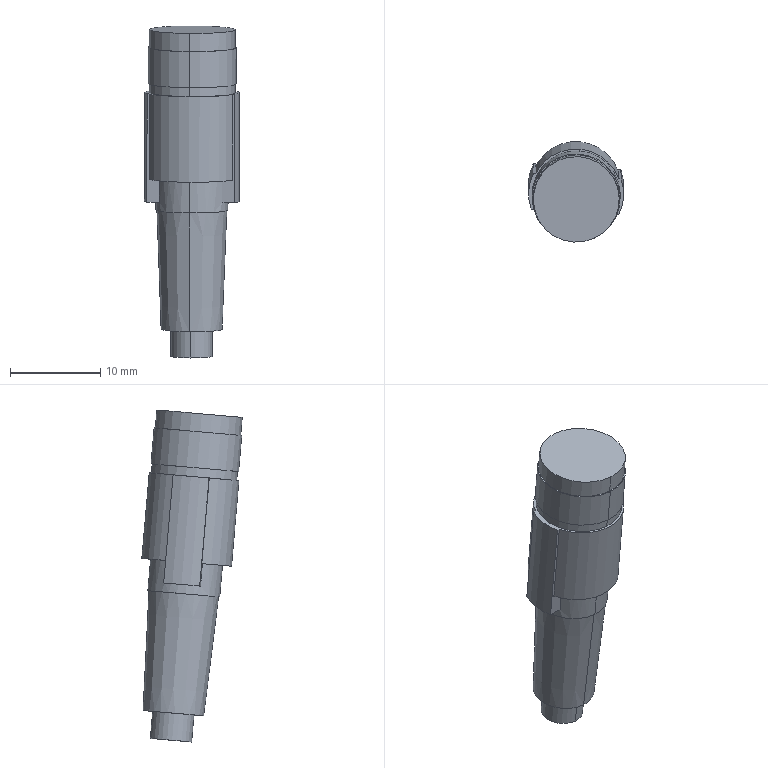Part | STEP file | 1_id1286_x_t | 1 solid | 31 faces | box 10.535 x 11.151 x 36.727 mm | volume 2077 mm3 | plane 15 | cylinder 14 | cone 2 | commonest cylinder face diameters 9.5 x4 4.6 x2 8 x2 9.75 x2 10 x2 10.508 x2